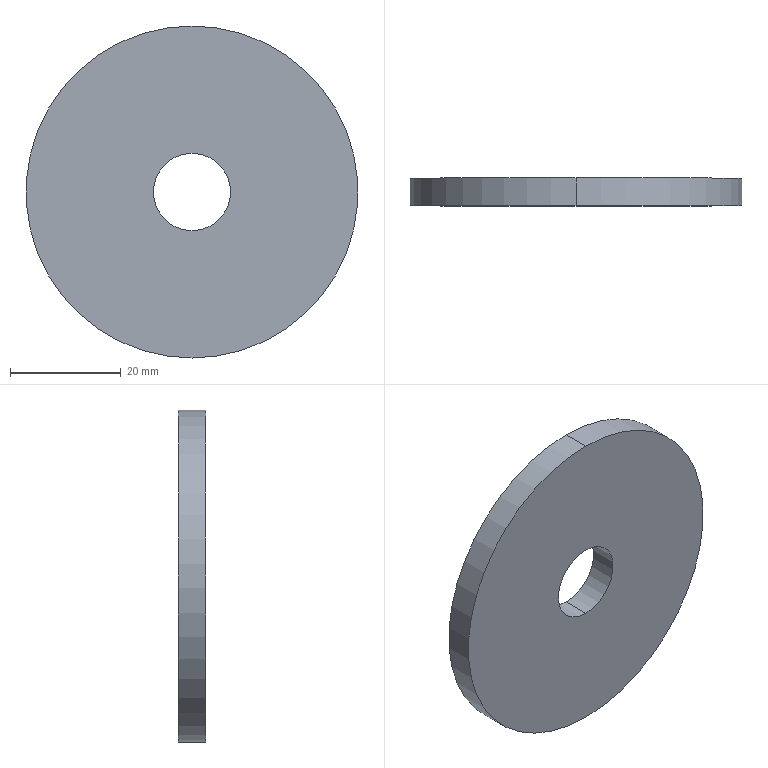Part | SolidWorks | features Extrusion 1 | 1 solid | 6 faces | box 60 x 5 x 60 mm | volume 13367 mm3 | cylinder 4 | plane 2 | commonest cylinder face diameters 14 x2 60 x2
STEP:
#1=CARTESIAN_POINT('',(0.,5.,-7.));
#2=VERTEX_POINT('',#1);
#3=CARTESIAN_POINT('',(0.,5.,7.));
#4=VERTEX_POINT('',#3);
#5=CARTESIAN_POINT('',(0.,5.,0.));
#6=DIRECTION('',(0.,1.,0.));
#7=DIRECTION('',(0.,0.,1.));
#8=AXIS2_PLACEMENT_3D('',#5,#6,#7);
#9=CIRCLE('',#8,7.);
#10=EDGE_CURVE('',#2,#4,#9,.T.);
#11=ORIENTED_EDGE('',*,*,#10,.T.);
#12=CARTESIAN_POINT('',(0.,0.,7.));
#13=VERTEX_POINT('',#12);
#14=CARTESIAN_POINT('',(0.,5.,7.));
#15=DIRECTION('',(0.,-1.,0.));
#16=VECTOR('',#15,1000.);
#17=LINE('',#14,#16);
#18=EDGE_CURVE('',#4,#13,#17,.T.);
#19=ORIENTED_EDGE('',*,*,#18,.T.);
#20=CARTESIAN_POINT('',(0.,0.,-7.));
#21=VERTEX_POINT('',#20);
#22=CARTESIAN_POINT('',(0.,0.,0.));
#23=DIRECTION('',(0.,1.,0.));
#24=DIRECTION('',(0.,0.,1.));
#25=AXIS2_PLACEMENT_3D('',#22,#23,#24);
#26=CIRCLE('',#25,7.);
#27=EDGE_CURVE('',#21,#13,#26,.T.);
#28=ORIENTED_EDGE('',*,*,#27,.F.);
#29=CARTESIAN_POINT('',(0.,5.,-7.));
#30=DIRECTION('',(0.,-1.,0.));
#31=VECTOR('',#30,1000.);
#32=LINE('',#29,#31);
#33=EDGE_CURVE('',#2,#21,#32,.T.);
#34=ORIENTED_EDGE('',*,*,#33,.F.);
#35=EDGE_LOOP('',(#11,#19,#28,#34));
#36=FACE_OUTER_BOUND('',#35,.T.);
#37=CARTESIAN_POINT('',(0.,5.,0.));
#38=DIRECTION('',(0.,-1.,0.));
#39=DIRECTION('',(0.,0.,-1.));
#40=AXIS2_PLACEMENT_3D('',#37,#38,#39);
#41=CYLINDRICAL_SURFACE('',#40,7.);
#42=ADVANCED_FACE('',(#36),#41,.F.);
#43=CARTESIAN_POINT('',(0.,5.,30.));
#44=VERTEX_POINT('',#43);
#45=CARTESIAN_POINT('',(0.,5.,-30.));
#46=VERTEX_POINT('',#45);
#47=CARTESIAN_POINT('',(0.,5.,0.));
#48=DIRECTION('',(0.,1.,0.));
#49=DIRECTION('',(0.,0.,1.));
#50=AXIS2_PLACEMENT_3D('',#47,#48,#49);
#51=CIRCLE('',#50,30.);
#52=EDGE_CURVE('',#44,#46,#51,.T.);
#53=ORIENTED_EDGE('',*,*,#52,.F.);
#54=CARTESIAN_POINT('',(0.,0.,30.));
#55=VERTEX_POINT('',#54);
#56=CARTESIAN_POINT('',(0.,5.,30.));
#57=DIRECTION('',(0.,-1.,0.));
#58=VECTOR('',#57,1000.);
#59=LINE('',#56,#58);
#60=EDGE_CURVE('',#44,#55,#59,.T.);
#61=ORIENTED_EDGE('',*,*,#60,.T.);
#62=CARTESIAN_POINT('',(0.,0.,-30.));
#63=VERTEX_POINT('',#62);
#64=CARTESIAN_POINT('',(0.,0.,0.));
#65=DIRECTION('',(0.,1.,0.));
#66=DIRECTION('',(0.,0.,1.));
#67=AXIS2_PLACEMENT_3D('',#64,#65,#66);
#68=CIRCLE('',#67,30.);
#69=EDGE_CURVE('',#55,#63,#68,.T.);
#70=ORIENTED_EDGE('',*,*,#69,.T.);
#71=CARTESIAN_POINT('',(0.,5.,-30.));
#72=DIRECTION('',(0.,-1.,0.));
#73=VECTOR('',#72,1000.);
#74=LINE('',#71,#73);
#75=EDGE_CURVE('',#46,#63,#74,.T.);
#76=ORIENTED_EDGE('',*,*,#75,.F.);
#77=EDGE_LOOP('',(#53,#61,#70,#76));
#78=FACE_OUTER_BOUND('',#77,.T.);
#79=CARTESIAN_POINT('',(0.,5.,0.));
#80=DIRECTION('',(0.,-1.,0.));
#81=DIRECTION('',(0.,0.,-1.));
#82=AXIS2_PLACEMENT_3D('',#79,#80,#81);
#83=CYLINDRICAL_SURFACE('',#82,30.);
#84=ADVANCED_FACE('',(#78),#83,.T.);
#85=CARTESIAN_POINT('',(0.,5.,0.));
#86=DIRECTION('',(0.,1.,0.));
#87=DIRECTION('',(0.,0.,1.));
#88=AXIS2_PLACEMENT_3D('',#85,#86,#87);
#89=CIRCLE('',#88,30.);
#90=EDGE_CURVE('',#46,#44,#89,.T.);
#91=ORIENTED_EDGE('',*,*,#90,.T.);
#92=ORIENTED_EDGE('',*,*,#52,.T.);
#93=EDGE_LOOP('',(#91,#92));
#94=FACE_OUTER_BOUND('',#93,.T.);
#95=ORIENTED_EDGE('',*,*,#10,.F.);
#96=CARTESIAN_POINT('',(0.,5.,0.));
#97=DIRECTION('',(0.,1.,0.));
#98=DIRECTION('',(0.,0.,1.));
#99=AXIS2_PLACEMENT_3D('',#96,#97,#98);
#100=CIRCLE('',#99,7.);
#101=EDGE_CURVE('',#4,#2,#100,.T.);
#102=ORIENTED_EDGE('',*,*,#101,.F.);
#103=EDGE_LOOP('',(#95,#102));
#104=FACE_BOUND('',#103,.T.);
#105=CARTESIAN_POINT('',(0.,5.,0.));
#106=DIRECTION('',(0.,1.,0.));
#107=DIRECTION('',(0.,0.,1.));
#108=AXIS2_PLACEMENT_3D('',#105,#106,#107);
#109=PLANE('',#108);
#110=ADVANCED_FACE('',(#94,#104),#109,.T.);
#111=CARTESIAN_POINT('',(0.,0.,0.));
#112=DIRECTION('',(0.,1.,0.));
#113=DIRECTION('',(0.,0.,1.));
#114=AXIS2_PLACEMENT_3D('',#111,#112,#113);
#115=CIRCLE('',#114,30.);
#116=EDGE_CURVE('',#63,#55,#115,.T.);
#117=ORIENTED_EDGE('',*,*,#116,.F.);
#118=ORIENTED_EDGE('',*,*,#69,.F.);
#119=EDGE_LOOP('',(#117,#118));
#120=FACE_OUTER_BOUND('',#119,.T.);
#121=ORIENTED_EDGE('',*,*,#27,.T.);
#122=CARTESIAN_POINT('',(0.,0.,0.));
#123=DIRECTION('',(0.,1.,0.));
#124=DIRECTION('',(0.,0.,1.));
#125=AXIS2_PLACEMENT_3D('',#122,#123,#124);
#126=CIRCLE('',#125,7.);
#127=EDGE_CURVE('',#13,#21,#126,.T.);
#128=ORIENTED_EDGE('',*,*,#127,.T.);
#129=EDGE_LOOP('',(#121,#128));
#130=FACE_BOUND('',#129,.T.);
#131=CARTESIAN_POINT('',(0.,0.,0.));
#132=DIRECTION('',(0.,1.,0.));
#133=DIRECTION('',(0.,0.,1.));
#134=AXIS2_PLACEMENT_3D('',#131,#132,#133);
#135=PLANE('',#134);
#136=ADVANCED_FACE('',(#120,#130),#135,.F.);
#137=ORIENTED_EDGE('',*,*,#60,.F.);
#138=ORIENTED_EDGE('',*,*,#90,.F.);
#139=ORIENTED_EDGE('',*,*,#75,.T.);
#140=ORIENTED_EDGE('',*,*,#116,.T.);
#141=EDGE_LOOP('',(#137,#138,#139,#140));
#142=FACE_OUTER_BOUND('',#141,.T.);
#143=CARTESIAN_POINT('',(0.,5.,0.));
#144=DIRECTION('',(0.,-1.,0.));
#145=DIRECTION('',(0.,0.,-1.));
#146=AXIS2_PLACEMENT_3D('',#143,#144,#145);
#147=CYLINDRICAL_SURFACE('',#146,30.);
#148=ADVANCED_FACE('',(#142),#147,.T.);
#149=ORIENTED_EDGE('',*,*,#18,.F.);
#150=ORIENTED_EDGE('',*,*,#101,.T.);
#151=ORIENTED_EDGE('',*,*,#33,.T.);
#152=ORIENTED_EDGE('',*,*,#127,.F.);
#153=EDGE_LOOP('',(#149,#150,#151,#152));
#154=FACE_OUTER_BOUND('',#153,.T.);
#155=CARTESIAN_POINT('',(0.,5.,0.));
#156=DIRECTION('',(0.,-1.,0.));
#157=DIRECTION('',(0.,0.,-1.));
#158=AXIS2_PLACEMENT_3D('',#155,#156,#157);
#159=CYLINDRICAL_SURFACE('',#158,7.);
#160=ADVANCED_FACE('',(#154),#159,.F.);
#161=CLOSED_SHELL('',(#42,#84,#110,#136,#148,#160));
#162=MANIFOLD_SOLID_BREP('',#161);
#163=CARTESIAN_POINT('',(0.,0.,0.));
#164=DIRECTION('',(0.,0.,1.));
#165=DIRECTION('',(1.,0.,0.));
#166=AXIS2_PLACEMENT_3D('',#163,#164,#165);
#167=(LENGTH_UNIT()NAMED_UNIT(*)SI_UNIT(.MILLI.,.METRE.));
#168=UNCERTAINTY_MEASURE_WITH_UNIT(LENGTH_MEASURE(0.00001),#167,'','');
#169=(NAMED_UNIT(*)PLANE_ANGLE_UNIT()SI_UNIT($,.RADIAN.));
#170=(NAMED_UNIT(*)SI_UNIT($,.STERADIAN.)SOLID_ANGLE_UNIT());
#171=(GEOMETRIC_REPRESENTATION_CONTEXT(3)GLOBAL_UNCERTAINTY_ASSIGNED_CONTEXT((#168))GLOBAL_UNIT_ASSIGNED_CONTEXT((#167,#169,#170))REPRESENTATION_CONTEXT('',''));
#172=ADVANCED_BREP_SHAPE_REPRESENTATION('',(#162,#166),#171);